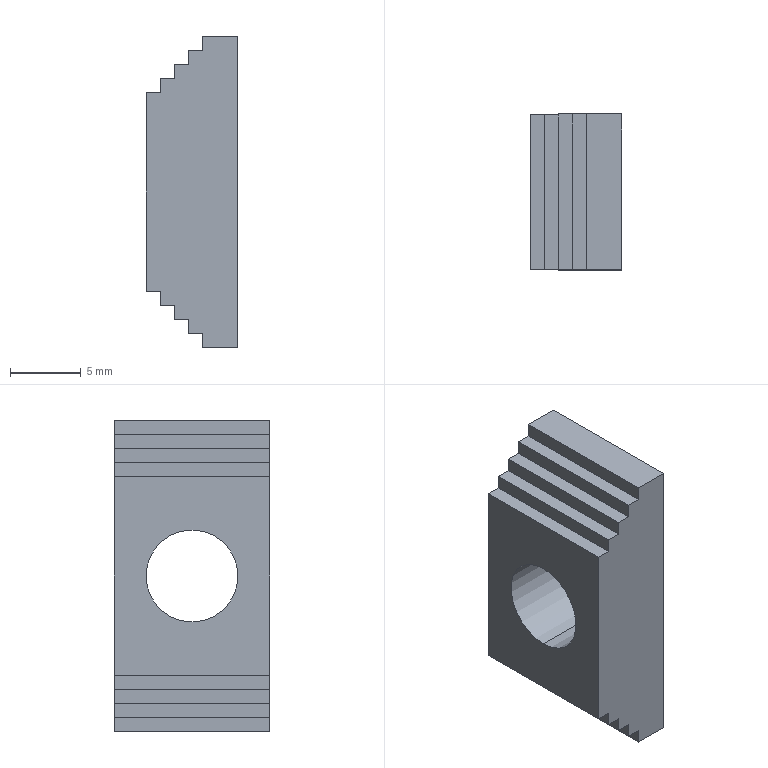Part | SolidWorks | features BaseBody 1 | 1 solid | 24 faces | box 6.5 x 11 x 22 mm | volume 1137 mm3 | plane 22 | cylinder 2 | commonest cylinder face diameters 6.5 x2
STEP:
#1=CARTESIAN_POINT('',(-38.513,101.396,43.5));
#2=VERTEX_POINT('',#1);
#3=CARTESIAN_POINT('',(-38.513,101.396,37.));
#4=VERTEX_POINT('',#3);
#5=CARTESIAN_POINT('',(-38.513,101.396,40.25));
#6=DIRECTION('',(-1.,0.,0.));
#7=DIRECTION('',(0.,0.,-1.));
#8=AXIS2_PLACEMENT_3D('',#5,#6,#7);
#9=CIRCLE('',#8,3.25);
#10=EDGE_CURVE('',#2,#4,#9,.T.);
#11=ORIENTED_EDGE('',*,*,#10,.T.);
#12=CARTESIAN_POINT('',(-32.013,101.396,37.));
#13=VERTEX_POINT('',#12);
#14=CARTESIAN_POINT('',(-38.513,101.396,37.));
#15=DIRECTION('',(1.,0.,0.));
#16=VECTOR('',#15,1000.);
#17=LINE('',#14,#16);
#18=EDGE_CURVE('',#4,#13,#17,.T.);
#19=ORIENTED_EDGE('',*,*,#18,.T.);
#20=CARTESIAN_POINT('',(-32.013,101.396,43.5));
#21=VERTEX_POINT('',#20);
#22=CARTESIAN_POINT('',(-32.013,101.396,40.25));
#23=DIRECTION('',(-1.,0.,0.));
#24=DIRECTION('',(0.,0.,-1.));
#25=AXIS2_PLACEMENT_3D('',#22,#23,#24);
#26=CIRCLE('',#25,3.25);
#27=EDGE_CURVE('',#21,#13,#26,.T.);
#28=ORIENTED_EDGE('',*,*,#27,.F.);
#29=CARTESIAN_POINT('',(-38.513,101.396,43.5));
#30=DIRECTION('',(1.,0.,0.));
#31=VECTOR('',#30,1000.);
#32=LINE('',#29,#31);
#33=EDGE_CURVE('',#2,#21,#32,.T.);
#34=ORIENTED_EDGE('',*,*,#33,.F.);
#35=EDGE_LOOP('',(#11,#19,#28,#34));
#36=FACE_OUTER_BOUND('',#35,.T.);
#37=CARTESIAN_POINT('',(-38.513,101.396,40.25));
#38=DIRECTION('',(1.,0.,0.));
#39=DIRECTION('',(0.,0.,1.));
#40=AXIS2_PLACEMENT_3D('',#37,#38,#39);
#41=CYLINDRICAL_SURFACE('',#40,3.25);
#42=ADVANCED_FACE('',(#36),#41,.F.);
#43=CARTESIAN_POINT('',(-34.513,106.896,51.25));
#44=VERTEX_POINT('',#43);
#45=CARTESIAN_POINT('',(-34.513,106.896,50.25));
#46=VERTEX_POINT('',#45);
#47=CARTESIAN_POINT('',(-34.513,106.896,50.25));
#48=DIRECTION('',(0.,0.,-1.));
#49=VECTOR('',#48,1000.);
#50=LINE('',#47,#49);
#51=EDGE_CURVE('',#44,#46,#50,.T.);
#52=ORIENTED_EDGE('',*,*,#51,.T.);
#53=CARTESIAN_POINT('',(-34.513,95.896,50.25));
#54=VERTEX_POINT('',#53);
#55=CARTESIAN_POINT('',(-34.513,95.896,50.25));
#56=DIRECTION('',(0.,1.,0.));
#57=VECTOR('',#56,1000.);
#58=LINE('',#55,#57);
#59=EDGE_CURVE('',#54,#46,#58,.T.);
#60=ORIENTED_EDGE('',*,*,#59,.F.);
#61=CARTESIAN_POINT('',(-34.513,95.896,51.25));
#62=VERTEX_POINT('',#61);
#63=CARTESIAN_POINT('',(-34.513,95.896,50.25));
#64=DIRECTION('',(0.,0.,-1.));
#65=VECTOR('',#64,1000.);
#66=LINE('',#63,#65);
#67=EDGE_CURVE('',#62,#54,#66,.T.);
#68=ORIENTED_EDGE('',*,*,#67,.F.);
#69=CARTESIAN_POINT('',(-34.513,95.896,51.25));
#70=DIRECTION('',(0.,1.,0.));
#71=VECTOR('',#70,1000.);
#72=LINE('',#69,#71);
#73=EDGE_CURVE('',#62,#44,#72,.T.);
#74=ORIENTED_EDGE('',*,*,#73,.T.);
#75=EDGE_LOOP('',(#52,#60,#68,#74));
#76=FACE_OUTER_BOUND('',#75,.T.);
#77=CARTESIAN_POINT('',(-34.513,95.896,50.25));
#78=DIRECTION('',(1.,0.,0.));
#79=DIRECTION('',(0.,0.,1.));
#80=AXIS2_PLACEMENT_3D('',#77,#78,#79);
#81=PLANE('',#80);
#82=ADVANCED_FACE('',(#76),#81,.F.);
#83=CARTESIAN_POINT('',(-35.513,106.896,50.25));
#84=VERTEX_POINT('',#83);
#85=CARTESIAN_POINT('',(-35.513,106.896,50.25));
#86=DIRECTION('',(-1.,0.,0.));
#87=VECTOR('',#86,1000.);
#88=LINE('',#85,#87);
#89=EDGE_CURVE('',#46,#84,#88,.T.);
#90=ORIENTED_EDGE('',*,*,#89,.T.);
#91=CARTESIAN_POINT('',(-35.513,95.896,50.25));
#92=VERTEX_POINT('',#91);
#93=CARTESIAN_POINT('',(-35.513,95.896,50.25));
#94=DIRECTION('',(0.,1.,0.));
#95=VECTOR('',#94,1000.);
#96=LINE('',#93,#95);
#97=EDGE_CURVE('',#92,#84,#96,.T.);
#98=ORIENTED_EDGE('',*,*,#97,.F.);
#99=CARTESIAN_POINT('',(-35.513,95.896,50.25));
#100=DIRECTION('',(-1.,0.,0.));
#101=VECTOR('',#100,1000.);
#102=LINE('',#99,#101);
#103=EDGE_CURVE('',#54,#92,#102,.T.);
#104=ORIENTED_EDGE('',*,*,#103,.F.);
#105=ORIENTED_EDGE('',*,*,#59,.T.);
#106=EDGE_LOOP('',(#90,#98,#104,#105));
#107=FACE_OUTER_BOUND('',#106,.T.);
#108=CARTESIAN_POINT('',(-35.513,95.896,50.25));
#109=DIRECTION('',(0.,0.,-1.));
#110=DIRECTION('',(-1.,0.,0.));
#111=AXIS2_PLACEMENT_3D('',#108,#109,#110);
#112=PLANE('',#111);
#113=ADVANCED_FACE('',(#107),#112,.F.);
#114=CARTESIAN_POINT('',(-35.513,106.896,49.25));
#115=VERTEX_POINT('',#114);
#116=CARTESIAN_POINT('',(-35.513,106.896,49.25));
#117=DIRECTION('',(0.,0.,-1.));
#118=VECTOR('',#117,1000.);
#119=LINE('',#116,#118);
#120=EDGE_CURVE('',#84,#115,#119,.T.);
#121=ORIENTED_EDGE('',*,*,#120,.T.);
#122=CARTESIAN_POINT('',(-35.513,95.896,49.25));
#123=VERTEX_POINT('',#122);
#124=CARTESIAN_POINT('',(-35.513,95.896,49.25));
#125=DIRECTION('',(0.,1.,0.));
#126=VECTOR('',#125,1000.);
#127=LINE('',#124,#126);
#128=EDGE_CURVE('',#123,#115,#127,.T.);
#129=ORIENTED_EDGE('',*,*,#128,.F.);
#130=CARTESIAN_POINT('',(-35.513,95.896,49.25));
#131=DIRECTION('',(0.,0.,-1.));
#132=VECTOR('',#131,1000.);
#133=LINE('',#130,#132);
#134=EDGE_CURVE('',#92,#123,#133,.T.);
#135=ORIENTED_EDGE('',*,*,#134,.F.);
#136=ORIENTED_EDGE('',*,*,#97,.T.);
#137=EDGE_LOOP('',(#121,#129,#135,#136));
#138=FACE_OUTER_BOUND('',#137,.T.);
#139=CARTESIAN_POINT('',(-35.513,95.896,49.25));
#140=DIRECTION('',(1.,0.,0.));
#141=DIRECTION('',(0.,0.,-1.));
#142=AXIS2_PLACEMENT_3D('',#139,#140,#141);
#143=PLANE('',#142);
#144=ADVANCED_FACE('',(#138),#143,.F.);
#145=CARTESIAN_POINT('',(-36.513,106.896,49.25));
#146=VERTEX_POINT('',#145);
#147=CARTESIAN_POINT('',(-36.513,106.896,49.25));
#148=DIRECTION('',(-1.,0.,0.));
#149=VECTOR('',#148,1000.);
#150=LINE('',#147,#149);
#151=EDGE_CURVE('',#115,#146,#150,.T.);
#152=ORIENTED_EDGE('',*,*,#151,.T.);
#153=CARTESIAN_POINT('',(-36.513,95.896,49.25));
#154=VERTEX_POINT('',#153);
#155=CARTESIAN_POINT('',(-36.513,95.896,49.25));
#156=DIRECTION('',(0.,1.,0.));
#157=VECTOR('',#156,1000.);
#158=LINE('',#155,#157);
#159=EDGE_CURVE('',#154,#146,#158,.T.);
#160=ORIENTED_EDGE('',*,*,#159,.F.);
#161=CARTESIAN_POINT('',(-36.513,95.896,49.25));
#162=DIRECTION('',(-1.,0.,0.));
#163=VECTOR('',#162,1000.);
#164=LINE('',#161,#163);
#165=EDGE_CURVE('',#123,#154,#164,.T.);
#166=ORIENTED_EDGE('',*,*,#165,.F.);
#167=ORIENTED_EDGE('',*,*,#128,.T.);
#168=EDGE_LOOP('',(#152,#160,#166,#167));
#169=FACE_OUTER_BOUND('',#168,.T.);
#170=CARTESIAN_POINT('',(-36.513,95.896,49.25));
#171=DIRECTION('',(0.,0.,-1.));
#172=DIRECTION('',(-1.,0.,0.));
#173=AXIS2_PLACEMENT_3D('',#170,#171,#172);
#174=PLANE('',#173);
#175=ADVANCED_FACE('',(#169),#174,.F.);
#176=CARTESIAN_POINT('',(-36.513,106.896,48.25));
#177=VERTEX_POINT('',#176);
#178=CARTESIAN_POINT('',(-36.513,106.896,48.25));
#179=DIRECTION('',(0.,0.,-1.));
#180=VECTOR('',#179,1000.);
#181=LINE('',#178,#180);
#182=EDGE_CURVE('',#146,#177,#181,.T.);
#183=ORIENTED_EDGE('',*,*,#182,.T.);
#184=CARTESIAN_POINT('',(-36.513,95.896,48.25));
#185=VERTEX_POINT('',#184);
#186=CARTESIAN_POINT('',(-36.513,95.896,48.25));
#187=DIRECTION('',(0.,1.,0.));
#188=VECTOR('',#187,1000.);
#189=LINE('',#186,#188);
#190=EDGE_CURVE('',#185,#177,#189,.T.);
#191=ORIENTED_EDGE('',*,*,#190,.F.);
#192=CARTESIAN_POINT('',(-36.513,95.896,48.25));
#193=DIRECTION('',(0.,0.,-1.));
#194=VECTOR('',#193,1000.);
#195=LINE('',#192,#194);
#196=EDGE_CURVE('',#154,#185,#195,.T.);
#197=ORIENTED_EDGE('',*,*,#196,.F.);
#198=ORIENTED_EDGE('',*,*,#159,.T.);
#199=EDGE_LOOP('',(#183,#191,#197,#198));
#200=FACE_OUTER_BOUND('',#199,.T.);
#201=CARTESIAN_POINT('',(-36.513,95.896,48.25));
#202=DIRECTION('',(1.,0.,0.));
#203=DIRECTION('',(0.,0.,-1.));
#204=AXIS2_PLACEMENT_3D('',#201,#202,#203);
#205=PLANE('',#204);
#206=ADVANCED_FACE('',(#200),#205,.F.);
#207=CARTESIAN_POINT('',(-37.513,106.896,48.25));
#208=VERTEX_POINT('',#207);
#209=CARTESIAN_POINT('',(-37.513,106.896,48.25));
#210=DIRECTION('',(-1.,0.,0.));
#211=VECTOR('',#210,1000.);
#212=LINE('',#209,#211);
#213=EDGE_CURVE('',#177,#208,#212,.T.);
#214=ORIENTED_EDGE('',*,*,#213,.T.);
#215=CARTESIAN_POINT('',(-37.513,95.896,48.25));
#216=VERTEX_POINT('',#215);
#217=CARTESIAN_POINT('',(-37.513,95.896,48.25));
#218=DIRECTION('',(0.,1.,0.));
#219=VECTOR('',#218,1000.);
#220=LINE('',#217,#219);
#221=EDGE_CURVE('',#216,#208,#220,.T.);
#222=ORIENTED_EDGE('',*,*,#221,.F.);
#223=CARTESIAN_POINT('',(-37.513,95.896,48.25));
#224=DIRECTION('',(-1.,0.,0.));
#225=VECTOR('',#224,1000.);
#226=LINE('',#223,#225);
#227=EDGE_CURVE('',#185,#216,#226,.T.);
#228=ORIENTED_EDGE('',*,*,#227,.F.);
#229=ORIENTED_EDGE('',*,*,#190,.T.);
#230=EDGE_LOOP('',(#214,#222,#228,#229));
#231=FACE_OUTER_BOUND('',#230,.T.);
#232=CARTESIAN_POINT('',(-37.513,95.896,48.25));
#233=DIRECTION('',(0.,0.,-1.));
#234=DIRECTION('',(-1.,0.,0.));
#235=AXIS2_PLACEMENT_3D('',#232,#233,#234);
#236=PLANE('',#235);
#237=ADVANCED_FACE('',(#231),#236,.F.);
#238=CARTESIAN_POINT('',(-37.513,106.896,47.25));
#239=VERTEX_POINT('',#238);
#240=CARTESIAN_POINT('',(-37.513,106.896,47.25));
#241=DIRECTION('',(0.,0.,-1.));
#242=VECTOR('',#241,1000.);
#243=LINE('',#240,#242);
#244=EDGE_CURVE('',#208,#239,#243,.T.);
#245=ORIENTED_EDGE('',*,*,#244,.T.);
#246=CARTESIAN_POINT('',(-37.513,95.896,47.25));
#247=VERTEX_POINT('',#246);
#248=CARTESIAN_POINT('',(-37.513,95.896,47.25));
#249=DIRECTION('',(0.,1.,0.));
#250=VECTOR('',#249,1000.);
#251=LINE('',#248,#250);
#252=EDGE_CURVE('',#247,#239,#251,.T.);
#253=ORIENTED_EDGE('',*,*,#252,.F.);
#254=CARTESIAN_POINT('',(-37.513,95.896,47.25));
#255=DIRECTION('',(0.,0.,-1.));
#256=VECTOR('',#255,1000.);
#257=LINE('',#254,#256);
#258=EDGE_CURVE('',#216,#247,#257,.T.);
#259=ORIENTED_EDGE('',*,*,#258,.F.);
#260=ORIENTED_EDGE('',*,*,#221,.T.);
#261=EDGE_LOOP('',(#245,#253,#259,#260));
#262=FACE_OUTER_BOUND('',#261,.T.);
#263=CARTESIAN_POINT('',(-37.513,95.896,47.25));
#264=DIRECTION('',(1.,0.,0.));
#265=DIRECTION('',(0.,0.,-1.));
#266=AXIS2_PLACEMENT_3D('',#263,#264,#265);
#267=PLANE('',#266);
#268=ADVANCED_FACE('',(#262),#267,.F.);
#269=CARTESIAN_POINT('',(-38.513,106.896,47.25));
#270=VERTEX_POINT('',#269);
#271=CARTESIAN_POINT('',(-38.513,106.896,47.25));
#272=DIRECTION('',(-1.,0.,0.));
#273=VECTOR('',#272,1000.);
#274=LINE('',#271,#273);
#275=EDGE_CURVE('',#239,#270,#274,.T.);
#276=ORIENTED_EDGE('',*,*,#275,.T.);
#277=CARTESIAN_POINT('',(-38.513,95.896,47.25));
#278=VERTEX_POINT('',#277);
#279=CARTESIAN_POINT('',(-38.513,95.896,47.25));
#280=DIRECTION('',(0.,1.,0.));
#281=VECTOR('',#280,1000.);
#282=LINE('',#279,#281);
#283=EDGE_CURVE('',#278,#270,#282,.T.);
#284=ORIENTED_EDGE('',*,*,#283,.F.);
#285=CARTESIAN_POINT('',(-38.513,95.896,47.25));
#286=DIRECTION('',(-1.,0.,0.));
#287=VECTOR('',#286,1000.);
#288=LINE('',#285,#287);
#289=EDGE_CURVE('',#247,#278,#288,.T.);
#290=ORIENTED_EDGE('',*,*,#289,.F.);
#291=ORIENTED_EDGE('',*,*,#252,.T.);
#292=EDGE_LOOP('',(#276,#284,#290,#291));
#293=FACE_OUTER_BOUND('',#292,.T.);
#294=CARTESIAN_POINT('',(-38.513,95.896,47.25));
#295=DIRECTION('',(0.,0.,-1.));
#296=DIRECTION('',(0.,-1.,0.));
#297=AXIS2_PLACEMENT_3D('',#294,#295,#296);
#298=PLANE('',#297);
#299=ADVANCED_FACE('',(#293),#298,.F.);
#300=CARTESIAN_POINT('',(-37.513,106.896,32.25));
#301=VERTEX_POINT('',#300);
#302=CARTESIAN_POINT('',(-36.513,106.896,32.25));
#303=VERTEX_POINT('',#302);
#304=CARTESIAN_POINT('',(-37.513,106.896,32.25));
#305=DIRECTION('',(1.,0.,0.));
#306=VECTOR('',#305,1000.);
#307=LINE('',#304,#306);
#308=EDGE_CURVE('',#301,#303,#307,.T.);
#309=ORIENTED_EDGE('',*,*,#308,.T.);
#310=CARTESIAN_POINT('',(-36.513,95.896,32.25));
#311=VERTEX_POINT('',#310);
#312=CARTESIAN_POINT('',(-36.513,95.896,32.25));
#313=DIRECTION('',(0.,1.,0.));
#314=VECTOR('',#313,1000.);
#315=LINE('',#312,#314);
#316=EDGE_CURVE('',#311,#303,#315,.T.);
#317=ORIENTED_EDGE('',*,*,#316,.F.);
#318=CARTESIAN_POINT('',(-37.513,95.896,32.25));
#319=VERTEX_POINT('',#318);
#320=CARTESIAN_POINT('',(-37.513,95.896,32.25));
#321=DIRECTION('',(1.,0.,0.));
#322=VECTOR('',#321,1000.);
#323=LINE('',#320,#322);
#324=EDGE_CURVE('',#319,#311,#323,.T.);
#325=ORIENTED_EDGE('',*,*,#324,.F.);
#326=CARTESIAN_POINT('',(-37.513,95.896,32.25));
#327=DIRECTION('',(0.,1.,0.));
#328=VECTOR('',#327,1000.);
#329=LINE('',#326,#328);
#330=EDGE_CURVE('',#319,#301,#329,.T.);
#331=ORIENTED_EDGE('',*,*,#330,.T.);
#332=EDGE_LOOP('',(#309,#317,#325,#331));
#333=FACE_OUTER_BOUND('',#332,.T.);
#334=CARTESIAN_POINT('',(-37.513,95.896,32.25));
#335=DIRECTION('',(0.,0.,1.));
#336=DIRECTION('',(1.,0.,0.));
#337=AXIS2_PLACEMENT_3D('',#334,#335,#336);
#338=PLANE('',#337);
#339=ADVANCED_FACE('',(#333),#338,.F.);
#340=CARTESIAN_POINT('',(-36.513,106.896,31.25));
#341=VERTEX_POINT('',#340);
#342=CARTESIAN_POINT('',(-36.513,106.896,32.25));
#343=DIRECTION('',(0.,0.,-1.));
#344=VECTOR('',#343,1000.);
#345=LINE('',#342,#344);
#346=EDGE_CURVE('',#303,#341,#345,.T.);
#347=ORIENTED_EDGE('',*,*,#346,.T.);
#348=CARTESIAN_POINT('',(-36.513,95.896,31.25));
#349=VERTEX_POINT('',#348);
#350=CARTESIAN_POINT('',(-36.513,95.896,31.25));
#351=DIRECTION('',(0.,1.,0.));
#352=VECTOR('',#351,1000.);
#353=LINE('',#350,#352);
#354=EDGE_CURVE('',#349,#341,#353,.T.);
#355=ORIENTED_EDGE('',*,*,#354,.F.);
#356=CARTESIAN_POINT('',(-36.513,95.896,32.25));
#357=DIRECTION('',(0.,0.,-1.));
#358=VECTOR('',#357,1000.);
#359=LINE('',#356,#358);
#360=EDGE_CURVE('',#311,#349,#359,.T.);
#361=ORIENTED_EDGE('',*,*,#360,.F.);
#362=ORIENTED_EDGE('',*,*,#316,.T.);
#363=EDGE_LOOP('',(#347,#355,#361,#362));
#364=FACE_OUTER_BOUND('',#363,.T.);
#365=CARTESIAN_POINT('',(-36.513,95.896,32.25));
#366=DIRECTION('',(1.,0.,0.));
#367=DIRECTION('',(0.,0.,-1.));
#368=AXIS2_PLACEMENT_3D('',#365,#366,#367);
#369=PLANE('',#368);
#370=ADVANCED_FACE('',(#364),#369,.F.);
#371=CARTESIAN_POINT('',(-35.513,106.896,31.25));
#372=VERTEX_POINT('',#371);
#373=CARTESIAN_POINT('',(-36.513,106.896,31.25));
#374=DIRECTION('',(1.,0.,0.));
#375=VECTOR('',#374,1000.);
#376=LINE('',#373,#375);
#377=EDGE_CURVE('',#341,#372,#376,.T.);
#378=ORIENTED_EDGE('',*,*,#377,.T.);
#379=CARTESIAN_POINT('',(-35.513,95.896,31.25));
#380=VERTEX_POINT('',#379);
#381=CARTESIAN_POINT('',(-35.513,95.896,31.25));
#382=DIRECTION('',(0.,1.,0.));
#383=VECTOR('',#382,1000.);
#384=LINE('',#381,#383);
#385=EDGE_CURVE('',#380,#372,#384,.T.);
#386=ORIENTED_EDGE('',*,*,#385,.F.);
#387=CARTESIAN_POINT('',(-36.513,95.896,31.25));
#388=DIRECTION('',(1.,0.,0.));
#389=VECTOR('',#388,1000.);
#390=LINE('',#387,#389);
#391=EDGE_CURVE('',#349,#380,#390,.T.);
#392=ORIENTED_EDGE('',*,*,#391,.F.);
#393=ORIENTED_EDGE('',*,*,#354,.T.);
#394=EDGE_LOOP('',(#378,#386,#392,#393));
#395=FACE_OUTER_BOUND('',#394,.T.);
#396=CARTESIAN_POINT('',(-36.513,95.896,31.25));
#397=DIRECTION('',(0.,0.,1.));
#398=DIRECTION('',(1.,0.,0.));
#399=AXIS2_PLACEMENT_3D('',#396,#397,#398);
#400=PLANE('',#399);
#401=ADVANCED_FACE('',(#395),#400,.F.);
#402=CARTESIAN_POINT('',(-35.513,106.896,30.25));
#403=VERTEX_POINT('',#402);
#404=CARTESIAN_POINT('',(-35.513,106.896,31.25));
#405=DIRECTION('',(0.,0.,-1.));
#406=VECTOR('',#405,1000.);
#407=LINE('',#404,#406);
#408=EDGE_CURVE('',#372,#403,#407,.T.);
#409=ORIENTED_EDGE('',*,*,#408,.T.);
#410=CARTESIAN_POINT('',(-35.513,95.896,30.25));
#411=VERTEX_POINT('',#410);
#412=CARTESIAN_POINT('',(-35.513,95.896,30.25));
#413=DIRECTION('',(0.,1.,0.));
#414=VECTOR('',#413,1000.);
#415=LINE('',#412,#414);
#416=EDGE_CURVE('',#411,#403,#415,.T.);
#417=ORIENTED_EDGE('',*,*,#416,.F.);
#418=CARTESIAN_POINT('',(-35.513,95.896,31.25));
#419=DIRECTION('',(0.,0.,-1.));
#420=VECTOR('',#419,1000.);
#421=LINE('',#418,#420);
#422=EDGE_CURVE('',#380,#411,#421,.T.);
#423=ORIENTED_EDGE('',*,*,#422,.F.);
#424=ORIENTED_EDGE('',*,*,#385,.T.);
#425=EDGE_LOOP('',(#409,#417,#423,#424));
#426=FACE_OUTER_BOUND('',#425,.T.);
#427=CARTESIAN_POINT('',(-35.513,95.896,31.25));
#428=DIRECTION('',(1.,0.,0.));
#429=DIRECTION('',(0.,0.,-1.));
#430=AXIS2_PLACEMENT_3D('',#427,#428,#429);
#431=PLANE('',#430);
#432=ADVANCED_FACE('',(#426),#431,.F.);
#433=CARTESIAN_POINT('',(-34.513,106.896,30.25));
#434=VERTEX_POINT('',#433);
#435=CARTESIAN_POINT('',(-35.513,106.896,30.25));
#436=DIRECTION('',(1.,0.,0.));
#437=VECTOR('',#436,1000.);
#438=LINE('',#435,#437);
#439=EDGE_CURVE('',#403,#434,#438,.T.);
#440=ORIENTED_EDGE('',*,*,#439,.T.);
#441=CARTESIAN_POINT('',(-34.513,95.896,30.25));
#442=VERTEX_POINT('',#441);
#443=CARTESIAN_POINT('',(-34.513,95.896,30.25));
#444=DIRECTION('',(0.,1.,0.));
#445=VECTOR('',#444,1000.);
#446=LINE('',#443,#445);
#447=EDGE_CURVE('',#442,#434,#446,.T.);
#448=ORIENTED_EDGE('',*,*,#447,.F.);
#449=CARTESIAN_POINT('',(-35.513,95.896,30.25));
#450=DIRECTION('',(1.,0.,0.));
#451=VECTOR('',#450,1000.);
#452=LINE('',#449,#451);
#453=EDGE_CURVE('',#411,#442,#452,.T.);
#454=ORIENTED_EDGE('',*,*,#453,.F.);
#455=ORIENTED_EDGE('',*,*,#416,.T.);
#456=EDGE_LOOP('',(#440,#448,#454,#455));
#457=FACE_OUTER_BOUND('',#456,.T.);
#458=CARTESIAN_POINT('',(-35.513,95.896,30.25));
#459=DIRECTION('',(0.,0.,1.));
#460=DIRECTION('',(1.,0.,0.));
#461=AXIS2_PLACEMENT_3D('',#458,#459,#460);
#462=PLANE('',#461);
#463=ADVANCED_FACE('',(#457),#462,.F.);
#464=CARTESIAN_POINT('',(-34.513,106.896,29.25));
#465=VERTEX_POINT('',#464);
#466=CARTESIAN_POINT('',(-34.513,106.896,30.25));
#467=DIRECTION('',(0.,0.,-1.));
#468=VECTOR('',#467,1000.);
#469=LINE('',#466,#468);
#470=EDGE_CURVE('',#434,#465,#469,.T.);
#471=ORIENTED_EDGE('',*,*,#470,.T.);
#472=CARTESIAN_POINT('',(-34.513,95.896,29.25));
#473=VERTEX_POINT('',#472);
#474=CARTESIAN_POINT('',(-34.513,95.896,29.25));
#475=DIRECTION('',(0.,1.,0.));
#476=VECTOR('',#475,1000.);
#477=LINE('',#474,#476);
#478=EDGE_CURVE('',#473,#465,#477,.T.);
#479=ORIENTED_EDGE('',*,*,#478,.F.);
#480=CARTESIAN_POINT('',(-34.513,95.896,30.25));
#481=DIRECTION('',(0.,0.,-1.));
#482=VECTOR('',#481,1000.);
#483=LINE('',#480,#482);
#484=EDGE_CURVE('',#442,#473,#483,.T.);
#485=ORIENTED_EDGE('',*,*,#484,.F.);
#486=ORIENTED_EDGE('',*,*,#447,.T.);
#487=EDGE_LOOP('',(#471,#479,#485,#486));
#488=FACE_OUTER_BOUND('',#487,.T.);
#489=CARTESIAN_POINT('',(-34.513,95.896,30.25));
#490=DIRECTION('',(1.,0.,0.));
#491=DIRECTION('',(0.,0.,-1.));
#492=AXIS2_PLACEMENT_3D('',#489,#490,#491);
#493=PLANE('',#492);
#494=ADVANCED_FACE('',(#488),#493,.F.);
#495=CARTESIAN_POINT('',(-38.513,106.896,33.25));
#496=VERTEX_POINT('',#495);
#497=CARTESIAN_POINT('',(-37.513,106.896,33.25));
#498=VERTEX_POINT('',#497);
#499=CARTESIAN_POINT('',(-38.513,106.896,33.25));
#500=DIRECTION('',(1.,0.,0.));
#501=VECTOR('',#500,1000.);
#502=LINE('',#499,#501);
#503=EDGE_CURVE('',#496,#498,#502,.T.);
#504=ORIENTED_EDGE('',*,*,#503,.T.);
#505=CARTESIAN_POINT('',(-37.513,95.896,33.25));
#506=VERTEX_POINT('',#505);
#507=CARTESIAN_POINT('',(-37.513,95.896,33.25));
#508=DIRECTION('',(0.,1.,0.));
#509=VECTOR('',#508,1000.);
#510=LINE('',#507,#509);
#511=EDGE_CURVE('',#506,#498,#510,.T.);
#512=ORIENTED_EDGE('',*,*,#511,.F.);
#513=CARTESIAN_POINT('',(-38.513,95.896,33.25));
#514=VERTEX_POINT('',#513);
#515=CARTESIAN_POINT('',(-38.513,95.896,33.25));
#516=DIRECTION('',(1.,0.,0.));
#517=VECTOR('',#516,1000.);
#518=LINE('',#515,#517);
#519=EDGE_CURVE('',#514,#506,#518,.T.);
#520=ORIENTED_EDGE('',*,*,#519,.F.);
#521=CARTESIAN_POINT('',(-38.513,95.896,33.25));
#522=DIRECTION('',(0.,1.,0.));
#523=VECTOR('',#522,1000.);
#524=LINE('',#521,#523);
#525=EDGE_CURVE('',#514,#496,#524,.T.);
#526=ORIENTED_EDGE('',*,*,#525,.T.);
#527=EDGE_LOOP('',(#504,#512,#520,#526));
#528=FACE_OUTER_BOUND('',#527,.T.);
#529=CARTESIAN_POINT('',(-38.513,95.896,33.25));
#530=DIRECTION('',(0.,0.,1.));
#531=DIRECTION('',(1.,0.,0.));
#532=AXIS2_PLACEMENT_3D('',#529,#530,#531);
#533=PLANE('',#532);
#534=ADVANCED_FACE('',(#528),#533,.F.);
#535=CARTESIAN_POINT('',(-37.513,106.896,33.25));
#536=DIRECTION('',(0.,0.,-1.));
#537=VECTOR('',#536,1000.);
#538=LINE('',#535,#537);
#539=EDGE_CURVE('',#498,#301,#538,.T.);
#540=ORIENTED_EDGE('',*,*,#539,.T.);
#541=ORIENTED_EDGE('',*,*,#330,.F.);
#542=CARTESIAN_POINT('',(-37.513,95.896,33.25));
#543=DIRECTION('',(0.,0.,-1.));
#544=VECTOR('',#543,1000.);
#545=LINE('',#542,#544);
#546=EDGE_CURVE('',#506,#319,#545,.T.);
#547=ORIENTED_EDGE('',*,*,#546,.F.);
#548=ORIENTED_EDGE('',*,*,#511,.T.);
#549=EDGE_LOOP('',(#540,#541,#547,#548));
#550=FACE_OUTER_BOUND('',#549,.T.);
#551=CARTESIAN_POINT('',(-37.513,95.896,33.25));
#552=DIRECTION('',(1.,0.,0.));
#553=DIRECTION('',(0.,0.,-1.));
#554=AXIS2_PLACEMENT_3D('',#551,#552,#553);
#555=PLANE('',#554);
#556=ADVANCED_FACE('',(#550),#555,.F.);
#557=ORIENTED_EDGE('',*,*,#18,.F.);
#558=CARTESIAN_POINT('',(-38.513,101.396,40.25));
#559=DIRECTION('',(-1.,0.,0.));
#560=DIRECTION('',(0.,0.,-1.));
#561=AXIS2_PLACEMENT_3D('',#558,#559,#560);
#562=CIRCLE('',#561,3.25);
#563=EDGE_CURVE('',#4,#2,#562,.T.);
#564=ORIENTED_EDGE('',*,*,#563,.T.);
#565=ORIENTED_EDGE('',*,*,#33,.T.);
#566=CARTESIAN_POINT('',(-32.013,101.396,40.25));
#567=DIRECTION('',(-1.,0.,0.));
#568=DIRECTION('',(0.,0.,-1.));
#569=AXIS2_PLACEMENT_3D('',#566,#567,#568);
#570=CIRCLE('',#569,3.25);
#571=EDGE_CURVE('',#13,#21,#570,.T.);
#572=ORIENTED_EDGE('',*,*,#571,.F.);
#573=EDGE_LOOP('',(#557,#564,#565,#572));
#574=FACE_OUTER_BOUND('',#573,.T.);
#575=CARTESIAN_POINT('',(-38.513,101.396,40.25));
#576=DIRECTION('',(1.,0.,0.));
#577=DIRECTION('',(0.,0.,1.));
#578=AXIS2_PLACEMENT_3D('',#575,#576,#577);
#579=CYLINDRICAL_SURFACE('',#578,3.25);
#580=ADVANCED_FACE('',(#574),#579,.F.);
#581=CARTESIAN_POINT('',(-32.013,106.896,51.25));
#582=VERTEX_POINT('',#581);
#583=CARTESIAN_POINT('',(-38.513,106.896,51.25));
#584=DIRECTION('',(1.,0.,0.));
#585=VECTOR('',#584,1000.);
#586=LINE('',#583,#585);
#587=EDGE_CURVE('',#44,#582,#586,.T.);
#588=ORIENTED_EDGE('',*,*,#587,.F.);
#589=ORIENTED_EDGE('',*,*,#73,.F.);
#590=CARTESIAN_POINT('',(-32.013,95.896,51.25));
#591=VERTEX_POINT('',#590);
#592=CARTESIAN_POINT('',(-38.513,95.896,51.25));
#593=DIRECTION('',(1.,0.,0.));
#594=VECTOR('',#593,1000.);
#595=LINE('',#592,#594);
#596=EDGE_CURVE('',#62,#591,#595,.T.);
#597=ORIENTED_EDGE('',*,*,#596,.T.);
#598=CARTESIAN_POINT('',(-32.013,95.896,51.25));
#599=DIRECTION('',(0.,1.,0.));
#600=VECTOR('',#599,1000.);
#601=LINE('',#598,#600);
#602=EDGE_CURVE('',#591,#582,#601,.T.);
#603=ORIENTED_EDGE('',*,*,#602,.T.);
#604=EDGE_LOOP('',(#588,#589,#597,#603));
#605=FACE_OUTER_BOUND('',#604,.T.);
#606=CARTESIAN_POINT('',(-38.513,95.896,51.25));
#607=DIRECTION('',(0.,0.,-1.));
#608=DIRECTION('',(-1.,0.,0.));
#609=AXIS2_PLACEMENT_3D('',#606,#607,#608);
#610=PLANE('',#609);
#611=ADVANCED_FACE('',(#605),#610,.F.);
#612=ORIENTED_EDGE('',*,*,#258,.T.);
#613=ORIENTED_EDGE('',*,*,#289,.T.);
#614=CARTESIAN_POINT('',(-38.513,95.896,51.25));
#615=DIRECTION('',(0.,0.,1.));
#616=VECTOR('',#615,1000.);
#617=LINE('',#614,#616);
#618=EDGE_CURVE('',#514,#278,#617,.T.);
#619=ORIENTED_EDGE('',*,*,#618,.F.);
#620=ORIENTED_EDGE('',*,*,#519,.T.);
#621=ORIENTED_EDGE('',*,*,#546,.T.);
#622=ORIENTED_EDGE('',*,*,#324,.T.);
#623=ORIENTED_EDGE('',*,*,#360,.T.);
#624=ORIENTED_EDGE('',*,*,#391,.T.);
#625=ORIENTED_EDGE('',*,*,#422,.T.);
#626=ORIENTED_EDGE('',*,*,#453,.T.);
#627=ORIENTED_EDGE('',*,*,#484,.T.);
#628=CARTESIAN_POINT('',(-32.013,95.896,29.25));
#629=VERTEX_POINT('',#628);
#630=CARTESIAN_POINT('',(-38.513,95.896,29.25));
#631=DIRECTION('',(1.,0.,0.));
#632=VECTOR('',#631,1000.);
#633=LINE('',#630,#632);
#634=EDGE_CURVE('',#473,#629,#633,.T.);
#635=ORIENTED_EDGE('',*,*,#634,.T.);
#636=CARTESIAN_POINT('',(-32.013,95.896,51.25));
#637=DIRECTION('',(0.,0.,1.));
#638=VECTOR('',#637,1000.);
#639=LINE('',#636,#638);
#640=EDGE_CURVE('',#629,#591,#639,.T.);
#641=ORIENTED_EDGE('',*,*,#640,.T.);
#642=ORIENTED_EDGE('',*,*,#596,.F.);
#643=ORIENTED_EDGE('',*,*,#67,.T.);
#644=ORIENTED_EDGE('',*,*,#103,.T.);
#645=ORIENTED_EDGE('',*,*,#134,.T.);
#646=ORIENTED_EDGE('',*,*,#165,.T.);
#647=ORIENTED_EDGE('',*,*,#196,.T.);
#648=ORIENTED_EDGE('',*,*,#227,.T.);
#649=EDGE_LOOP('',(#612,#613,#619,#620,#621,#622,#623,#624,#625,#626,#627,#635,#641,#642,#643,#644,#645,#646,#647,#648));
#650=FACE_OUTER_BOUND('',#649,.T.);
#651=CARTESIAN_POINT('',(-38.513,95.896,51.25));
#652=DIRECTION('',(0.,1.,0.));
#653=DIRECTION('',(0.,0.,-1.));
#654=AXIS2_PLACEMENT_3D('',#651,#652,#653);
#655=PLANE('',#654);
#656=ADVANCED_FACE('',(#650),#655,.F.);
#657=ORIENTED_EDGE('',*,*,#634,.F.);
#658=ORIENTED_EDGE('',*,*,#478,.T.);
#659=CARTESIAN_POINT('',(-32.013,106.896,29.25));
#660=VERTEX_POINT('',#659);
#661=CARTESIAN_POINT('',(-38.513,106.896,29.25));
#662=DIRECTION('',(1.,0.,0.));
#663=VECTOR('',#662,1000.);
#664=LINE('',#661,#663);
#665=EDGE_CURVE('',#465,#660,#664,.T.);
#666=ORIENTED_EDGE('',*,*,#665,.T.);
#667=CARTESIAN_POINT('',(-32.013,95.896,29.25));
#668=DIRECTION('',(0.,-1.,0.));
#669=VECTOR('',#668,1000.);
#670=LINE('',#667,#669);
#671=EDGE_CURVE('',#660,#629,#670,.T.);
#672=ORIENTED_EDGE('',*,*,#671,.T.);
#673=EDGE_LOOP('',(#657,#658,#666,#672));
#674=FACE_OUTER_BOUND('',#673,.T.);
#675=CARTESIAN_POINT('',(-38.513,95.896,29.25));
#676=DIRECTION('',(0.,0.,1.));
#677=DIRECTION('',(0.,-1.,0.));
#678=AXIS2_PLACEMENT_3D('',#675,#676,#677);
#679=PLANE('',#678);
#680=ADVANCED_FACE('',(#674),#679,.F.);
#681=CARTESIAN_POINT('',(-38.513,106.896,51.25));
#682=DIRECTION('',(0.,0.,-1.));
#683=VECTOR('',#682,1000.);
#684=LINE('',#681,#683);
#685=EDGE_CURVE('',#270,#496,#684,.T.);
#686=ORIENTED_EDGE('',*,*,#685,.F.);
#687=ORIENTED_EDGE('',*,*,#275,.F.);
#688=ORIENTED_EDGE('',*,*,#244,.F.);
#689=ORIENTED_EDGE('',*,*,#213,.F.);
#690=ORIENTED_EDGE('',*,*,#182,.F.);
#691=ORIENTED_EDGE('',*,*,#151,.F.);
#692=ORIENTED_EDGE('',*,*,#120,.F.);
#693=ORIENTED_EDGE('',*,*,#89,.F.);
#694=ORIENTED_EDGE('',*,*,#51,.F.);
#695=ORIENTED_EDGE('',*,*,#587,.T.);
#696=CARTESIAN_POINT('',(-32.013,106.896,51.25));
#697=DIRECTION('',(0.,0.,-1.));
#698=VECTOR('',#697,1000.);
#699=LINE('',#696,#698);
#700=EDGE_CURVE('',#582,#660,#699,.T.);
#701=ORIENTED_EDGE('',*,*,#700,.T.);
#702=ORIENTED_EDGE('',*,*,#665,.F.);
#703=ORIENTED_EDGE('',*,*,#470,.F.);
#704=ORIENTED_EDGE('',*,*,#439,.F.);
#705=ORIENTED_EDGE('',*,*,#408,.F.);
#706=ORIENTED_EDGE('',*,*,#377,.F.);
#707=ORIENTED_EDGE('',*,*,#346,.F.);
#708=ORIENTED_EDGE('',*,*,#308,.F.);
#709=ORIENTED_EDGE('',*,*,#539,.F.);
#710=ORIENTED_EDGE('',*,*,#503,.F.);
#711=EDGE_LOOP('',(#686,#687,#688,#689,#690,#691,#692,#693,#694,#695,#701,#702,#703,#704,#705,#706,#707,#708,#709,#710));
#712=FACE_OUTER_BOUND('',#711,.T.);
#713=CARTESIAN_POINT('',(-38.513,106.896,51.25));
#714=DIRECTION('',(0.,-1.,0.));
#715=DIRECTION('',(-1.,0.,0.));
#716=AXIS2_PLACEMENT_3D('',#713,#714,#715);
#717=PLANE('',#716);
#718=ADVANCED_FACE('',(#712),#717,.F.);
#719=ORIENTED_EDGE('',*,*,#27,.T.);
#720=ORIENTED_EDGE('',*,*,#571,.T.);
#721=EDGE_LOOP('',(#719,#720));
#722=FACE_BOUND('',#721,.T.);
#723=ORIENTED_EDGE('',*,*,#700,.F.);
#724=ORIENTED_EDGE('',*,*,#602,.F.);
#725=ORIENTED_EDGE('',*,*,#640,.F.);
#726=ORIENTED_EDGE('',*,*,#671,.F.);
#727=EDGE_LOOP('',(#723,#724,#725,#726));
#728=FACE_OUTER_BOUND('',#727,.T.);
#729=CARTESIAN_POINT('',(-32.013,106.896,29.25));
#730=DIRECTION('',(1.,0.,0.));
#731=DIRECTION('',(0.,0.,-1.));
#732=AXIS2_PLACEMENT_3D('',#729,#730,#731);
#733=PLANE('',#732);
#734=ADVANCED_FACE('',(#722,#728),#733,.T.);
#735=ORIENTED_EDGE('',*,*,#10,.F.);
#736=ORIENTED_EDGE('',*,*,#563,.F.);
#737=EDGE_LOOP('',(#735,#736));
#738=FACE_BOUND('',#737,.T.);
#739=ORIENTED_EDGE('',*,*,#618,.T.);
#740=ORIENTED_EDGE('',*,*,#283,.T.);
#741=ORIENTED_EDGE('',*,*,#685,.T.);
#742=ORIENTED_EDGE('',*,*,#525,.F.);
#743=EDGE_LOOP('',(#739,#740,#741,#742));
#744=FACE_OUTER_BOUND('',#743,.T.);
#745=CARTESIAN_POINT('',(-38.513,106.896,29.25));
#746=DIRECTION('',(1.,0.,0.));
#747=DIRECTION('',(0.,0.,-1.));
#748=AXIS2_PLACEMENT_3D('',#745,#746,#747);
#749=PLANE('',#748);
#750=ADVANCED_FACE('',(#738,#744),#749,.F.);
#751=CLOSED_SHELL('',(#42,#82,#113,#144,#175,#206,#237,#268,#299,#339,#370,#401,#432,#463,#494,#534,#556,#580,#611,#656,#680,#718,#734,#750));
#752=MANIFOLD_SOLID_BREP('',#751);
#753=CARTESIAN_POINT('',(0.,0.,0.));
#754=DIRECTION('',(0.,0.,1.));
#755=DIRECTION('',(1.,0.,0.));
#756=AXIS2_PLACEMENT_3D('',#753,#754,#755);
#757=(LENGTH_UNIT()NAMED_UNIT(*)SI_UNIT(.MILLI.,.METRE.));
#758=UNCERTAINTY_MEASURE_WITH_UNIT(LENGTH_MEASURE(0.00001),#757,'','');
#759=(NAMED_UNIT(*)PLANE_ANGLE_UNIT()SI_UNIT($,.RADIAN.));
#760=(NAMED_UNIT(*)SI_UNIT($,.STERADIAN.)SOLID_ANGLE_UNIT());
#761=(GEOMETRIC_REPRESENTATION_CONTEXT(3)GLOBAL_UNCERTAINTY_ASSIGNED_CONTEXT((#758))GLOBAL_UNIT_ASSIGNED_CONTEXT((#757,#759,#760))REPRESENTATION_CONTEXT('',''));
#762=ADVANCED_BREP_SHAPE_REPRESENTATION('',(#752,#756),#761);